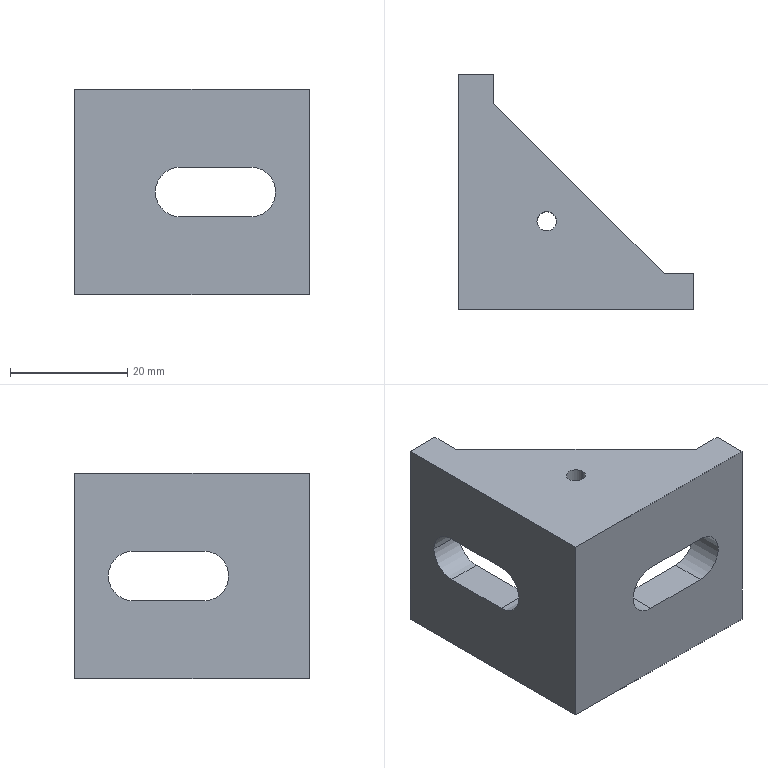Part | STEP file | PN_0039 (4040A foot bracket) | 1 solid | 26 faces | box 40 x 40 x 35 mm | volume 17755 mm3 | plane 16 | cylinder 10 | commonest cylinder face diameters 8.5 x6 3.3 x4